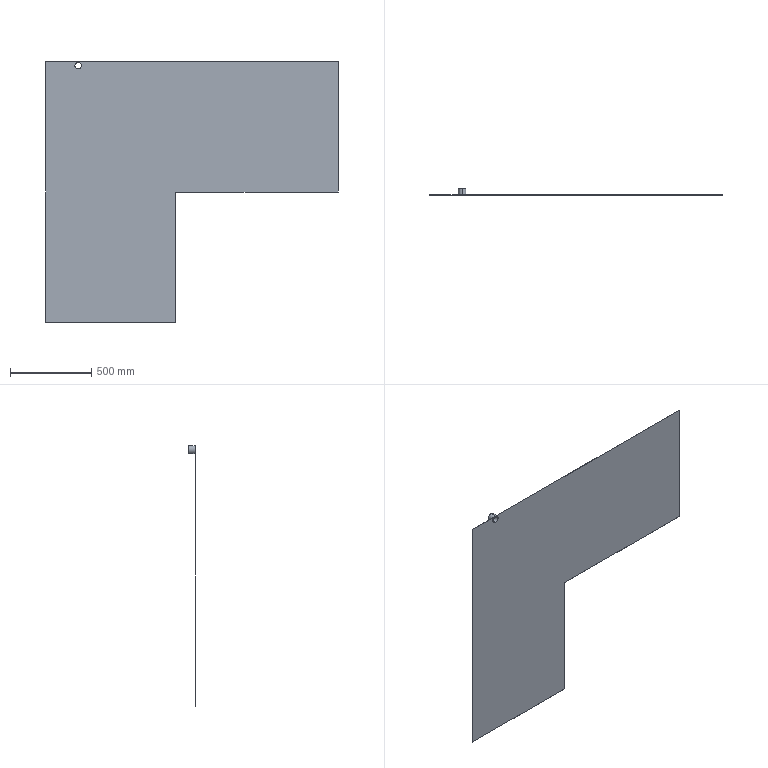Part | SolidWorks | features ICE 2, Extrusion 1 | 1 solid | 13 faces | box 1800 x 40 x 1600 mm | volume 2097397 mm3 | plane 9 | cylinder 4 | commonest cylinder face diameters 40 x2 47 x2
STEP:
#1=CARTESIAN_POINT('',(-700.,40.,800.));
#2=VERTEX_POINT('',#1);
#3=CARTESIAN_POINT('',(-700.,40.,753.));
#4=VERTEX_POINT('',#3);
#5=CARTESIAN_POINT('',(-700.,40.,776.5));
#6=DIRECTION('',(0.,1.,0.));
#7=DIRECTION('',(0.,0.,1.));
#8=AXIS2_PLACEMENT_3D('',#5,#6,#7);
#9=CIRCLE('',#8,23.5);
#10=EDGE_CURVE('',#2,#4,#9,.T.);
#11=ORIENTED_EDGE('',*,*,#10,.F.);
#12=CARTESIAN_POINT('',(-700.,1.,800.));
#13=VERTEX_POINT('',#12);
#14=CARTESIAN_POINT('',(-700.,40.,800.));
#15=DIRECTION('',(0.,-1.,0.));
#16=VECTOR('',#15,1000.);
#17=LINE('',#14,#16);
#18=EDGE_CURVE('',#2,#13,#17,.T.);
#19=ORIENTED_EDGE('',*,*,#18,.T.);
#20=CARTESIAN_POINT('',(-700.,1.,753.));
#21=VERTEX_POINT('',#20);
#22=CARTESIAN_POINT('',(-700.,1.,776.5));
#23=DIRECTION('',(0.,1.,0.));
#24=DIRECTION('',(0.,0.,1.));
#25=AXIS2_PLACEMENT_3D('',#22,#23,#24);
#26=CIRCLE('',#25,23.5);
#27=EDGE_CURVE('',#13,#21,#26,.T.);
#28=ORIENTED_EDGE('',*,*,#27,.T.);
#29=CARTESIAN_POINT('',(-700.,40.,753.));
#30=DIRECTION('',(0.,-1.,0.));
#31=VECTOR('',#30,1000.);
#32=LINE('',#29,#31);
#33=EDGE_CURVE('',#4,#21,#32,.T.);
#34=ORIENTED_EDGE('',*,*,#33,.F.);
#35=EDGE_LOOP('',(#11,#19,#28,#34));
#36=FACE_OUTER_BOUND('',#35,.T.);
#37=CARTESIAN_POINT('',(-700.,40.,776.5));
#38=DIRECTION('',(0.,-1.,0.));
#39=DIRECTION('',(0.,0.,-1.));
#40=AXIS2_PLACEMENT_3D('',#37,#38,#39);
#41=CYLINDRICAL_SURFACE('',#40,23.5);
#42=ADVANCED_FACE('',(#36),#41,.T.);
#43=CARTESIAN_POINT('',(-700.,0.,756.5));
#44=VERTEX_POINT('',#43);
#45=CARTESIAN_POINT('',(-700.,0.,796.5));
#46=VERTEX_POINT('',#45);
#47=CARTESIAN_POINT('',(-700.,0.,776.5));
#48=DIRECTION('',(0.,1.,0.));
#49=DIRECTION('',(0.,0.,1.));
#50=AXIS2_PLACEMENT_3D('',#47,#48,#49);
#51=CIRCLE('',#50,20.);
#52=EDGE_CURVE('',#44,#46,#51,.T.);
#53=ORIENTED_EDGE('',*,*,#52,.F.);
#54=CARTESIAN_POINT('',(-700.,40.,756.5));
#55=VERTEX_POINT('',#54);
#56=CARTESIAN_POINT('',(-700.,0.,756.5));
#57=DIRECTION('',(0.,1.,0.));
#58=VECTOR('',#57,1000.);
#59=LINE('',#56,#58);
#60=EDGE_CURVE('',#44,#55,#59,.T.);
#61=ORIENTED_EDGE('',*,*,#60,.T.);
#62=CARTESIAN_POINT('',(-700.,40.,796.5));
#63=VERTEX_POINT('',#62);
#64=CARTESIAN_POINT('',(-700.,40.,776.5));
#65=DIRECTION('',(0.,1.,0.));
#66=DIRECTION('',(0.,0.,1.));
#67=AXIS2_PLACEMENT_3D('',#64,#65,#66);
#68=CIRCLE('',#67,20.);
#69=EDGE_CURVE('',#55,#63,#68,.T.);
#70=ORIENTED_EDGE('',*,*,#69,.T.);
#71=CARTESIAN_POINT('',(-700.,0.,796.5));
#72=DIRECTION('',(0.,1.,0.));
#73=VECTOR('',#72,1000.);
#74=LINE('',#71,#73);
#75=EDGE_CURVE('',#46,#63,#74,.T.);
#76=ORIENTED_EDGE('',*,*,#75,.F.);
#77=EDGE_LOOP('',(#53,#61,#70,#76));
#78=FACE_OUTER_BOUND('',#77,.T.);
#79=CARTESIAN_POINT('',(-700.,0.,776.5));
#80=DIRECTION('',(0.,1.,0.));
#81=DIRECTION('',(0.,0.,1.));
#82=AXIS2_PLACEMENT_3D('',#79,#80,#81);
#83=CYLINDRICAL_SURFACE('',#82,20.);
#84=ADVANCED_FACE('',(#78),#83,.F.);
#85=CARTESIAN_POINT('',(-100.,0.,0.));
#86=VERTEX_POINT('',#85);
#87=CARTESIAN_POINT('',(-100.,0.,-800.));
#88=VERTEX_POINT('',#87);
#89=CARTESIAN_POINT('',(-100.,0.,-800.));
#90=DIRECTION('',(0.,0.,-1.));
#91=VECTOR('',#90,1000.);
#92=LINE('',#89,#91);
#93=EDGE_CURVE('',#86,#88,#92,.T.);
#94=ORIENTED_EDGE('',*,*,#93,.T.);
#95=CARTESIAN_POINT('',(-100.,1.,-800.));
#96=VERTEX_POINT('',#95);
#97=CARTESIAN_POINT('',(-100.,1.,-800.));
#98=DIRECTION('',(0.,-1.,0.));
#99=VECTOR('',#98,1000.);
#100=LINE('',#97,#99);
#101=EDGE_CURVE('',#96,#88,#100,.T.);
#102=ORIENTED_EDGE('',*,*,#101,.F.);
#103=CARTESIAN_POINT('',(-100.,1.,0.));
#104=VERTEX_POINT('',#103);
#105=CARTESIAN_POINT('',(-100.,1.,-800.));
#106=DIRECTION('',(0.,0.,-1.));
#107=VECTOR('',#106,1000.);
#108=LINE('',#105,#107);
#109=EDGE_CURVE('',#104,#96,#108,.T.);
#110=ORIENTED_EDGE('',*,*,#109,.F.);
#111=CARTESIAN_POINT('',(-100.,1.,0.));
#112=DIRECTION('',(0.,-1.,0.));
#113=VECTOR('',#112,1000.);
#114=LINE('',#111,#113);
#115=EDGE_CURVE('',#104,#86,#114,.T.);
#116=ORIENTED_EDGE('',*,*,#115,.T.);
#117=EDGE_LOOP('',(#94,#102,#110,#116));
#118=FACE_OUTER_BOUND('',#117,.T.);
#119=CARTESIAN_POINT('',(-100.,1.,-800.));
#120=DIRECTION('',(-1.,0.,0.));
#121=DIRECTION('',(0.,0.,1.));
#122=AXIS2_PLACEMENT_3D('',#119,#120,#121);
#123=PLANE('',#122);
#124=ADVANCED_FACE('',(#118),#123,.F.);
#125=CARTESIAN_POINT('',(-900.,0.,-800.));
#126=VERTEX_POINT('',#125);
#127=CARTESIAN_POINT('',(-900.,0.,-800.));
#128=DIRECTION('',(-1.,0.,0.));
#129=VECTOR('',#128,1000.);
#130=LINE('',#127,#129);
#131=EDGE_CURVE('',#88,#126,#130,.T.);
#132=ORIENTED_EDGE('',*,*,#131,.T.);
#133=CARTESIAN_POINT('',(-900.,1.,-800.));
#134=VERTEX_POINT('',#133);
#135=CARTESIAN_POINT('',(-900.,1.,-800.));
#136=DIRECTION('',(0.,-1.,0.));
#137=VECTOR('',#136,1000.);
#138=LINE('',#135,#137);
#139=EDGE_CURVE('',#134,#126,#138,.T.);
#140=ORIENTED_EDGE('',*,*,#139,.F.);
#141=CARTESIAN_POINT('',(-900.,1.,-800.));
#142=DIRECTION('',(-1.,0.,0.));
#143=VECTOR('',#142,1000.);
#144=LINE('',#141,#143);
#145=EDGE_CURVE('',#96,#134,#144,.T.);
#146=ORIENTED_EDGE('',*,*,#145,.F.);
#147=ORIENTED_EDGE('',*,*,#101,.T.);
#148=EDGE_LOOP('',(#132,#140,#146,#147));
#149=FACE_OUTER_BOUND('',#148,.T.);
#150=CARTESIAN_POINT('',(-900.,1.,-800.));
#151=DIRECTION('',(0.,0.,1.));
#152=DIRECTION('',(1.,0.,0.));
#153=AXIS2_PLACEMENT_3D('',#150,#151,#152);
#154=PLANE('',#153);
#155=ADVANCED_FACE('',(#149),#154,.F.);
#156=CARTESIAN_POINT('',(-900.,0.,800.));
#157=VERTEX_POINT('',#156);
#158=CARTESIAN_POINT('',(-900.,0.,800.));
#159=DIRECTION('',(0.,0.,1.));
#160=VECTOR('',#159,1000.);
#161=LINE('',#158,#160);
#162=EDGE_CURVE('',#126,#157,#161,.T.);
#163=ORIENTED_EDGE('',*,*,#162,.T.);
#164=CARTESIAN_POINT('',(-900.,1.,800.));
#165=VERTEX_POINT('',#164);
#166=CARTESIAN_POINT('',(-900.,1.,800.));
#167=DIRECTION('',(0.,-1.,0.));
#168=VECTOR('',#167,1000.);
#169=LINE('',#166,#168);
#170=EDGE_CURVE('',#165,#157,#169,.T.);
#171=ORIENTED_EDGE('',*,*,#170,.F.);
#172=CARTESIAN_POINT('',(-900.,1.,800.));
#173=DIRECTION('',(0.,0.,1.));
#174=VECTOR('',#173,1000.);
#175=LINE('',#172,#174);
#176=EDGE_CURVE('',#134,#165,#175,.T.);
#177=ORIENTED_EDGE('',*,*,#176,.F.);
#178=ORIENTED_EDGE('',*,*,#139,.T.);
#179=EDGE_LOOP('',(#163,#171,#177,#178));
#180=FACE_OUTER_BOUND('',#179,.T.);
#181=CARTESIAN_POINT('',(-900.,1.,800.));
#182=DIRECTION('',(1.,0.,0.));
#183=DIRECTION('',(0.,0.,-1.));
#184=AXIS2_PLACEMENT_3D('',#181,#182,#183);
#185=PLANE('',#184);
#186=ADVANCED_FACE('',(#180),#185,.F.);
#187=CARTESIAN_POINT('',(900.,0.,800.));
#188=VERTEX_POINT('',#187);
#189=CARTESIAN_POINT('',(-900.,0.,800.));
#190=DIRECTION('',(1.,0.,0.));
#191=VECTOR('',#190,1000.);
#192=LINE('',#189,#191);
#193=EDGE_CURVE('',#157,#188,#192,.T.);
#194=ORIENTED_EDGE('',*,*,#193,.T.);
#195=CARTESIAN_POINT('',(900.,1.,800.));
#196=VERTEX_POINT('',#195);
#197=CARTESIAN_POINT('',(900.,1.,800.));
#198=DIRECTION('',(0.,-1.,0.));
#199=VECTOR('',#198,1000.);
#200=LINE('',#197,#199);
#201=EDGE_CURVE('',#196,#188,#200,.T.);
#202=ORIENTED_EDGE('',*,*,#201,.F.);
#203=CARTESIAN_POINT('',(-900.,1.,800.));
#204=DIRECTION('',(1.,0.,0.));
#205=VECTOR('',#204,1000.);
#206=LINE('',#203,#205);
#207=EDGE_CURVE('',#13,#196,#206,.T.);
#208=ORIENTED_EDGE('',*,*,#207,.F.);
#209=CARTESIAN_POINT('',(-900.,1.,800.));
#210=DIRECTION('',(1.,0.,0.));
#211=VECTOR('',#210,1000.);
#212=LINE('',#209,#211);
#213=EDGE_CURVE('',#165,#13,#212,.T.);
#214=ORIENTED_EDGE('',*,*,#213,.F.);
#215=ORIENTED_EDGE('',*,*,#170,.T.);
#216=EDGE_LOOP('',(#194,#202,#208,#214,#215));
#217=FACE_OUTER_BOUND('',#216,.T.);
#218=CARTESIAN_POINT('',(-900.,1.,800.));
#219=DIRECTION('',(0.,0.,-1.));
#220=DIRECTION('',(-1.,0.,0.));
#221=AXIS2_PLACEMENT_3D('',#218,#219,#220);
#222=PLANE('',#221);
#223=ADVANCED_FACE('',(#217),#222,.F.);
#224=CARTESIAN_POINT('',(900.,0.,0.));
#225=VERTEX_POINT('',#224);
#226=CARTESIAN_POINT('',(900.,0.,800.));
#227=DIRECTION('',(0.,0.,-1.));
#228=VECTOR('',#227,1000.);
#229=LINE('',#226,#228);
#230=EDGE_CURVE('',#188,#225,#229,.T.);
#231=ORIENTED_EDGE('',*,*,#230,.T.);
#232=CARTESIAN_POINT('',(900.,1.,0.));
#233=VERTEX_POINT('',#232);
#234=CARTESIAN_POINT('',(900.,1.,0.));
#235=DIRECTION('',(0.,-1.,0.));
#236=VECTOR('',#235,1000.);
#237=LINE('',#234,#236);
#238=EDGE_CURVE('',#233,#225,#237,.T.);
#239=ORIENTED_EDGE('',*,*,#238,.F.);
#240=CARTESIAN_POINT('',(900.,1.,800.));
#241=DIRECTION('',(0.,0.,-1.));
#242=VECTOR('',#241,1000.);
#243=LINE('',#240,#242);
#244=EDGE_CURVE('',#196,#233,#243,.T.);
#245=ORIENTED_EDGE('',*,*,#244,.F.);
#246=ORIENTED_EDGE('',*,*,#201,.T.);
#247=EDGE_LOOP('',(#231,#239,#245,#246));
#248=FACE_OUTER_BOUND('',#247,.T.);
#249=CARTESIAN_POINT('',(900.,1.,800.));
#250=DIRECTION('',(-1.,0.,0.));
#251=DIRECTION('',(0.,0.,1.));
#252=AXIS2_PLACEMENT_3D('',#249,#250,#251);
#253=PLANE('',#252);
#254=ADVANCED_FACE('',(#248),#253,.F.);
#255=CARTESIAN_POINT('',(-100.,0.,0.));
#256=DIRECTION('',(-1.,0.,0.));
#257=VECTOR('',#256,1000.);
#258=LINE('',#255,#257);
#259=EDGE_CURVE('',#225,#86,#258,.T.);
#260=ORIENTED_EDGE('',*,*,#259,.T.);
#261=ORIENTED_EDGE('',*,*,#115,.F.);
#262=CARTESIAN_POINT('',(0.,1.,0.));
#263=DIRECTION('',(-1.,0.,0.));
#264=VECTOR('',#263,1000.);
#265=LINE('',#262,#264);
#266=EDGE_CURVE('',#233,#104,#265,.T.);
#267=ORIENTED_EDGE('',*,*,#266,.F.);
#268=ORIENTED_EDGE('',*,*,#238,.T.);
#269=EDGE_LOOP('',(#260,#261,#267,#268));
#270=FACE_OUTER_BOUND('',#269,.T.);
#271=CARTESIAN_POINT('',(-100.,1.,0.));
#272=DIRECTION('',(0.,0.,1.));
#273=DIRECTION('',(1.,0.,0.));
#274=AXIS2_PLACEMENT_3D('',#271,#272,#273);
#275=PLANE('',#274);
#276=ADVANCED_FACE('',(#270),#275,.F.);
#277=ORIENTED_EDGE('',*,*,#213,.T.);
#278=CARTESIAN_POINT('',(-700.,1.,776.5));
#279=DIRECTION('',(0.,1.,0.));
#280=DIRECTION('',(0.,0.,1.));
#281=AXIS2_PLACEMENT_3D('',#278,#279,#280);
#282=CIRCLE('',#281,23.5);
#283=EDGE_CURVE('',#21,#13,#282,.T.);
#284=ORIENTED_EDGE('',*,*,#283,.F.);
#285=ORIENTED_EDGE('',*,*,#27,.F.);
#286=ORIENTED_EDGE('',*,*,#207,.T.);
#287=ORIENTED_EDGE('',*,*,#244,.T.);
#288=ORIENTED_EDGE('',*,*,#266,.T.);
#289=ORIENTED_EDGE('',*,*,#109,.T.);
#290=ORIENTED_EDGE('',*,*,#145,.T.);
#291=ORIENTED_EDGE('',*,*,#176,.T.);
#292=EDGE_LOOP('',(#277,#284,#285,#286,#287,#288,#289,#290,#291));
#293=FACE_OUTER_BOUND('',#292,.T.);
#294=CARTESIAN_POINT('',(0.,1.,0.));
#295=DIRECTION('',(0.,1.,0.));
#296=DIRECTION('',(0.,0.,1.));
#297=AXIS2_PLACEMENT_3D('',#294,#295,#296);
#298=PLANE('',#297);
#299=ADVANCED_FACE('',(#293),#298,.T.);
#300=CARTESIAN_POINT('',(-700.,0.,776.5));
#301=DIRECTION('',(0.,1.,0.));
#302=DIRECTION('',(0.,0.,1.));
#303=AXIS2_PLACEMENT_3D('',#300,#301,#302);
#304=CIRCLE('',#303,20.);
#305=EDGE_CURVE('',#46,#44,#304,.T.);
#306=ORIENTED_EDGE('',*,*,#305,.T.);
#307=ORIENTED_EDGE('',*,*,#52,.T.);
#308=EDGE_LOOP('',(#306,#307));
#309=FACE_BOUND('',#308,.T.);
#310=ORIENTED_EDGE('',*,*,#93,.F.);
#311=ORIENTED_EDGE('',*,*,#259,.F.);
#312=ORIENTED_EDGE('',*,*,#230,.F.);
#313=ORIENTED_EDGE('',*,*,#193,.F.);
#314=ORIENTED_EDGE('',*,*,#162,.F.);
#315=ORIENTED_EDGE('',*,*,#131,.F.);
#316=EDGE_LOOP('',(#310,#311,#312,#313,#314,#315));
#317=FACE_OUTER_BOUND('',#316,.T.);
#318=CARTESIAN_POINT('',(0.,0.,0.));
#319=DIRECTION('',(0.,1.,0.));
#320=DIRECTION('',(0.,0.,1.));
#321=AXIS2_PLACEMENT_3D('',#318,#319,#320);
#322=PLANE('',#321);
#323=ADVANCED_FACE('',(#309,#317),#322,.F.);
#324=ORIENTED_EDGE('',*,*,#60,.F.);
#325=ORIENTED_EDGE('',*,*,#305,.F.);
#326=ORIENTED_EDGE('',*,*,#75,.T.);
#327=CARTESIAN_POINT('',(-700.,40.,776.5));
#328=DIRECTION('',(0.,1.,0.));
#329=DIRECTION('',(0.,0.,1.));
#330=AXIS2_PLACEMENT_3D('',#327,#328,#329);
#331=CIRCLE('',#330,20.);
#332=EDGE_CURVE('',#63,#55,#331,.T.);
#333=ORIENTED_EDGE('',*,*,#332,.T.);
#334=EDGE_LOOP('',(#324,#325,#326,#333));
#335=FACE_OUTER_BOUND('',#334,.T.);
#336=CARTESIAN_POINT('',(-700.,0.,776.5));
#337=DIRECTION('',(0.,1.,0.));
#338=DIRECTION('',(0.,0.,1.));
#339=AXIS2_PLACEMENT_3D('',#336,#337,#338);
#340=CYLINDRICAL_SURFACE('',#339,20.);
#341=ADVANCED_FACE('',(#335),#340,.F.);
#342=CARTESIAN_POINT('',(-700.,40.,776.5));
#343=DIRECTION('',(0.,1.,0.));
#344=DIRECTION('',(0.,0.,1.));
#345=AXIS2_PLACEMENT_3D('',#342,#343,#344);
#346=CIRCLE('',#345,23.5);
#347=EDGE_CURVE('',#4,#2,#346,.T.);
#348=ORIENTED_EDGE('',*,*,#347,.T.);
#349=ORIENTED_EDGE('',*,*,#10,.T.);
#350=EDGE_LOOP('',(#348,#349));
#351=FACE_OUTER_BOUND('',#350,.T.);
#352=ORIENTED_EDGE('',*,*,#332,.F.);
#353=ORIENTED_EDGE('',*,*,#69,.F.);
#354=EDGE_LOOP('',(#352,#353));
#355=FACE_BOUND('',#354,.T.);
#356=CARTESIAN_POINT('',(-700.,40.,776.5));
#357=DIRECTION('',(0.,1.,0.));
#358=DIRECTION('',(0.,0.,1.));
#359=AXIS2_PLACEMENT_3D('',#356,#357,#358);
#360=PLANE('',#359);
#361=ADVANCED_FACE('',(#351,#355),#360,.T.);
#362=ORIENTED_EDGE('',*,*,#18,.F.);
#363=ORIENTED_EDGE('',*,*,#347,.F.);
#364=ORIENTED_EDGE('',*,*,#33,.T.);
#365=ORIENTED_EDGE('',*,*,#283,.T.);
#366=EDGE_LOOP('',(#362,#363,#364,#365));
#367=FACE_OUTER_BOUND('',#366,.T.);
#368=CARTESIAN_POINT('',(-700.,40.,776.5));
#369=DIRECTION('',(0.,-1.,0.));
#370=DIRECTION('',(0.,0.,-1.));
#371=AXIS2_PLACEMENT_3D('',#368,#369,#370);
#372=CYLINDRICAL_SURFACE('',#371,23.5);
#373=ADVANCED_FACE('',(#367),#372,.T.);
#374=CLOSED_SHELL('',(#42,#84,#124,#155,#186,#223,#254,#276,#299,#323,#341,#361,#373));
#375=MANIFOLD_SOLID_BREP('',#374);
#376=CARTESIAN_POINT('',(0.,0.,0.));
#377=DIRECTION('',(0.,0.,1.));
#378=DIRECTION('',(1.,0.,0.));
#379=AXIS2_PLACEMENT_3D('',#376,#377,#378);
#380=(LENGTH_UNIT()NAMED_UNIT(*)SI_UNIT(.MILLI.,.METRE.));
#381=UNCERTAINTY_MEASURE_WITH_UNIT(LENGTH_MEASURE(0.00001),#380,'','');
#382=(NAMED_UNIT(*)PLANE_ANGLE_UNIT()SI_UNIT($,.RADIAN.));
#383=(NAMED_UNIT(*)SI_UNIT($,.STERADIAN.)SOLID_ANGLE_UNIT());
#384=(GEOMETRIC_REPRESENTATION_CONTEXT(3)GLOBAL_UNCERTAINTY_ASSIGNED_CONTEXT((#381))GLOBAL_UNIT_ASSIGNED_CONTEXT((#380,#382,#383))REPRESENTATION_CONTEXT('',''));
#385=ADVANCED_BREP_SHAPE_REPRESENTATION('',(#375,#379),#384);